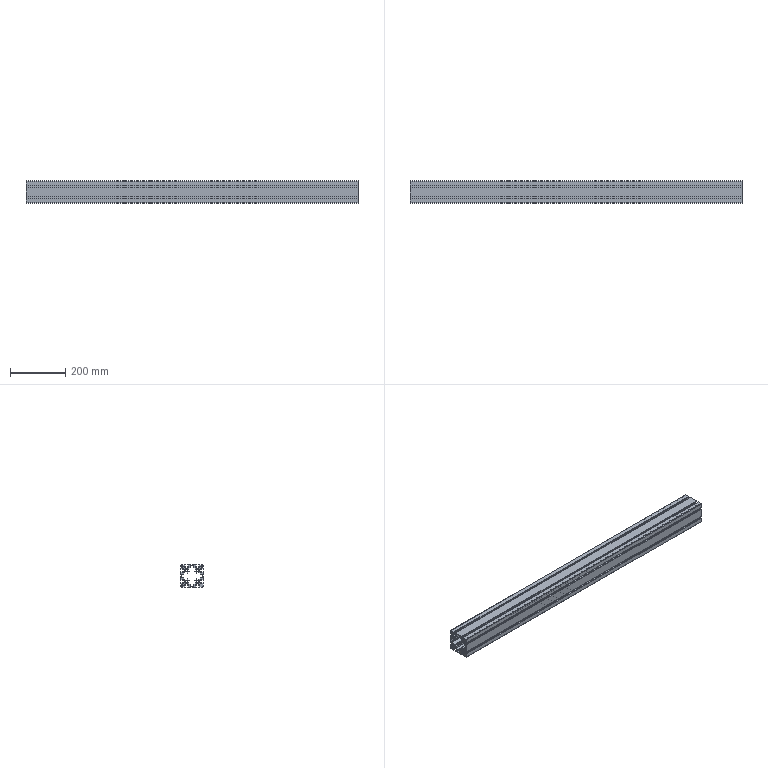Part | NX | 1 solid | 165 faces | box 1200 x 80 x 80 mm | volume 2780754 mm3 | plane 146 | cylinder 19 | commonest cylinder face diameters 2 x8 3 x4 6.8 x4 6 x3